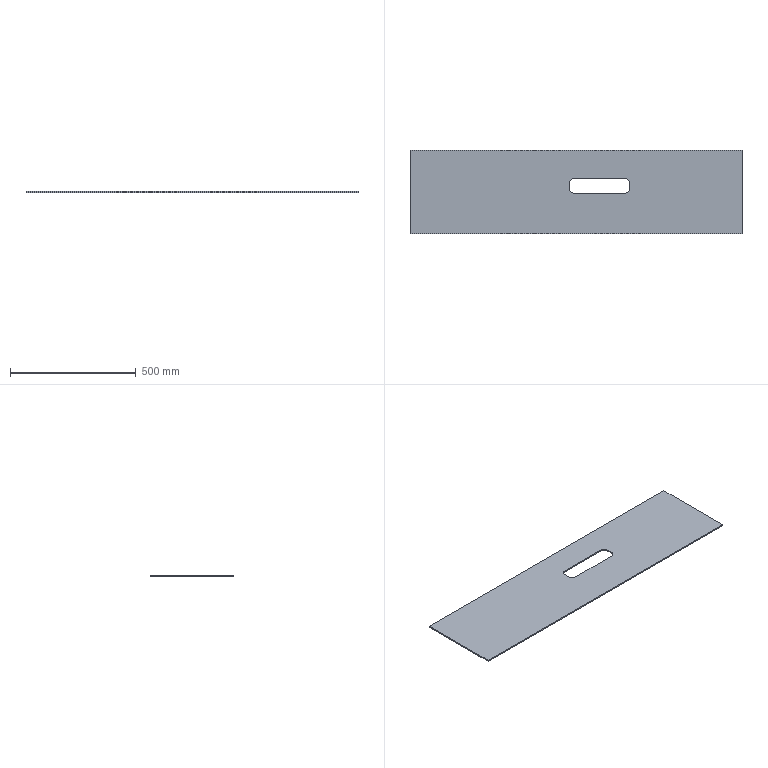Part | STEP file | 1 solid | 14 faces | box 1318 x 331 x 5 mm | volume 2111007 mm3 | plane 10 | cylinder 4 | commonest cylinder face diameters 40 x4
STEP:
#1=CARTESIAN_POINT('',(0.,0.,0.));
#2=DIRECTION('',(0.,0.,1.));
#3=DIRECTION('',(1.,0.,0.));
#4=AXIS2_PLACEMENT_3D('',#1,#2,#3);
#5=CARTESIAN_POINT('',(-7.,1028.,0.));
#6=VERTEX_POINT('',#5);
#7=CARTESIAN_POINT('',(193.,1028.,0.));
#8=VERTEX_POINT('',#7);
#9=CARTESIAN_POINT('',(-7.,1028.,0.));
#10=DIRECTION('',(1.,0.,0.));
#11=VECTOR('',#10,1.);
#12=LINE('',#9,#11);
#13=CARTESIAN_POINT('',(0.,0.,0.));
#14=DIRECTION('',(0.,0.,1.));
#15=DIRECTION('',(1.,0.,0.));
#16=AXIS2_PLACEMENT_3D('',#13,#14,#15);
#17=PLANE('',#16);
#18=CARTESIAN_POINT('',(-7.,1028.));
#19=DIRECTION('',(1.,0.));
#20=VECTOR('',#19,1.);
#21=LINE('',#18,#20);
#22=(GEOMETRIC_REPRESENTATION_CONTEXT(2)PARAMETRIC_REPRESENTATION_CONTEXT()REPRESENTATION_CONTEXT('',''));
#23=DEFINITIONAL_REPRESENTATION('',(#21),#22);
#24=PCURVE('',#17,#23);
#25=CARTESIAN_POINT('',(-7.,1028.,5.));
#26=DIRECTION('',(0.,-1.,0.));
#27=DIRECTION('',(0.,0.,-1.));
#28=AXIS2_PLACEMENT_3D('',#25,#26,#27);
#29=PLANE('',#28);
#30=CARTESIAN_POINT('',(5.,0.));
#31=DIRECTION('',(0.,1.));
#32=VECTOR('',#31,1.);
#33=LINE('',#30,#32);
#34=(GEOMETRIC_REPRESENTATION_CONTEXT(2)PARAMETRIC_REPRESENTATION_CONTEXT()REPRESENTATION_CONTEXT('',''));
#35=DEFINITIONAL_REPRESENTATION('',(#33),#34);
#36=PCURVE('',#29,#35);
#37=SURFACE_CURVE('',#12,(#24,#36),.PCURVE_S1.);
#38=EDGE_CURVE('',#6,#8,#37,.T.);
#39=ORIENTED_EDGE('',*,*,#38,.F.);
#40=CARTESIAN_POINT('',(-27.,1008.,0.));
#41=VERTEX_POINT('',#40);
#42=CARTESIAN_POINT('',(-7.,1008.,0.));
#43=DIRECTION('',(0.,0.,1.));
#44=DIRECTION('',(-1.,0.,0.));
#45=AXIS2_PLACEMENT_3D('',#42,#43,#44);
#46=CIRCLE('',#45,20.);
#47=CARTESIAN_POINT('',(-7.,1008.));
#48=DIRECTION('',(-1.,0.));
#49=AXIS2_PLACEMENT_2D('',#47,#48);
#50=CIRCLE('',#49,20.);
#51=(GEOMETRIC_REPRESENTATION_CONTEXT(2)PARAMETRIC_REPRESENTATION_CONTEXT()REPRESENTATION_CONTEXT('',''));
#52=DEFINITIONAL_REPRESENTATION('',(#50),#51);
#53=PCURVE('',#17,#52);
#54=CARTESIAN_POINT('',(-7.,1008.,5.));
#55=DIRECTION('',(0.,0.,-1.));
#56=DIRECTION('',(-1.,0.,0.));
#57=AXIS2_PLACEMENT_3D('',#54,#55,#56);
#58=CYLINDRICAL_SURFACE('',#57,20.);
#59=CARTESIAN_POINT('',(6.283,5.));
#60=DIRECTION('',(-1.,0.));
#61=VECTOR('',#60,1.);
#62=LINE('',#59,#61);
#63=(GEOMETRIC_REPRESENTATION_CONTEXT(2)PARAMETRIC_REPRESENTATION_CONTEXT()REPRESENTATION_CONTEXT('',''));
#64=DEFINITIONAL_REPRESENTATION('',(#62),#63);
#65=PCURVE('',#58,#64);
#66=SURFACE_CURVE('',#46,(#53,#65),.PCURVE_S1.);
#67=EDGE_CURVE('',#6,#41,#66,.T.);
#68=ORIENTED_EDGE('',*,*,#67,.T.);
#69=CARTESIAN_POINT('',(-27.,988.,0.));
#70=VERTEX_POINT('',#69);
#71=CARTESIAN_POINT('',(-27.,988.,0.));
#72=DIRECTION('',(0.,1.,0.));
#73=VECTOR('',#72,1.);
#74=LINE('',#71,#73);
#75=CARTESIAN_POINT('',(-27.,988.));
#76=DIRECTION('',(0.,1.));
#77=VECTOR('',#76,1.);
#78=LINE('',#75,#77);
#79=(GEOMETRIC_REPRESENTATION_CONTEXT(2)PARAMETRIC_REPRESENTATION_CONTEXT()REPRESENTATION_CONTEXT('',''));
#80=DEFINITIONAL_REPRESENTATION('',(#78),#79);
#81=PCURVE('',#17,#80);
#82=CARTESIAN_POINT('',(-27.,988.,5.));
#83=DIRECTION('',(1.,0.,0.));
#84=DIRECTION('',(0.,1.,0.));
#85=AXIS2_PLACEMENT_3D('',#82,#83,#84);
#86=PLANE('',#85);
#87=CARTESIAN_POINT('',(0.,-5.));
#88=DIRECTION('',(1.,0.));
#89=VECTOR('',#88,1.);
#90=LINE('',#87,#89);
#91=(GEOMETRIC_REPRESENTATION_CONTEXT(2)PARAMETRIC_REPRESENTATION_CONTEXT()REPRESENTATION_CONTEXT('',''));
#92=DEFINITIONAL_REPRESENTATION('',(#90),#91);
#93=PCURVE('',#86,#92);
#94=SURFACE_CURVE('',#74,(#81,#93),.PCURVE_S1.);
#95=EDGE_CURVE('',#70,#41,#94,.T.);
#96=ORIENTED_EDGE('',*,*,#95,.F.);
#97=CARTESIAN_POINT('',(-7.,968.,0.));
#98=VERTEX_POINT('',#97);
#99=CARTESIAN_POINT('',(-7.,988.,0.));
#100=DIRECTION('',(0.,0.,1.));
#101=DIRECTION('',(-1.,0.,0.));
#102=AXIS2_PLACEMENT_3D('',#99,#100,#101);
#103=CIRCLE('',#102,20.);
#104=CARTESIAN_POINT('',(-7.,988.));
#105=DIRECTION('',(-1.,0.));
#106=AXIS2_PLACEMENT_2D('',#104,#105);
#107=CIRCLE('',#106,20.);
#108=(GEOMETRIC_REPRESENTATION_CONTEXT(2)PARAMETRIC_REPRESENTATION_CONTEXT()REPRESENTATION_CONTEXT('',''));
#109=DEFINITIONAL_REPRESENTATION('',(#107),#108);
#110=PCURVE('',#17,#109);
#111=CARTESIAN_POINT('',(-7.,988.,5.));
#112=DIRECTION('',(0.,0.,-1.));
#113=DIRECTION('',(-1.,0.,0.));
#114=AXIS2_PLACEMENT_3D('',#111,#112,#113);
#115=CYLINDRICAL_SURFACE('',#114,20.);
#116=CARTESIAN_POINT('',(6.283,5.));
#117=DIRECTION('',(-1.,0.));
#118=VECTOR('',#117,1.);
#119=LINE('',#116,#118);
#120=(GEOMETRIC_REPRESENTATION_CONTEXT(2)PARAMETRIC_REPRESENTATION_CONTEXT()REPRESENTATION_CONTEXT('',''));
#121=DEFINITIONAL_REPRESENTATION('',(#119),#120);
#122=PCURVE('',#115,#121);
#123=SURFACE_CURVE('',#103,(#110,#122),.PCURVE_S1.);
#124=EDGE_CURVE('',#70,#98,#123,.T.);
#125=ORIENTED_EDGE('',*,*,#124,.T.);
#126=CARTESIAN_POINT('',(193.,968.,0.));
#127=VERTEX_POINT('',#126);
#128=CARTESIAN_POINT('',(-7.,968.,0.));
#129=DIRECTION('',(-1.,0.,0.));
#130=VECTOR('',#129,1.);
#131=LINE('',#128,#130);
#132=CARTESIAN_POINT('',(-7.,968.));
#133=DIRECTION('',(-1.,0.));
#134=VECTOR('',#133,1.);
#135=LINE('',#132,#134);
#136=(GEOMETRIC_REPRESENTATION_CONTEXT(2)PARAMETRIC_REPRESENTATION_CONTEXT()REPRESENTATION_CONTEXT('',''));
#137=DEFINITIONAL_REPRESENTATION('',(#135),#136);
#138=PCURVE('',#17,#137);
#139=CARTESIAN_POINT('',(-7.,968.,5.));
#140=DIRECTION('',(0.,1.,0.));
#141=DIRECTION('',(1.,0.,0.));
#142=AXIS2_PLACEMENT_3D('',#139,#140,#141);
#143=PLANE('',#142);
#144=CARTESIAN_POINT('',(0.,5.));
#145=DIRECTION('',(-1.,0.));
#146=VECTOR('',#145,1.);
#147=LINE('',#144,#146);
#148=(GEOMETRIC_REPRESENTATION_CONTEXT(2)PARAMETRIC_REPRESENTATION_CONTEXT()REPRESENTATION_CONTEXT('',''));
#149=DEFINITIONAL_REPRESENTATION('',(#147),#148);
#150=PCURVE('',#143,#149);
#151=SURFACE_CURVE('',#131,(#138,#150),.PCURVE_S1.);
#152=EDGE_CURVE('',#127,#98,#151,.T.);
#153=ORIENTED_EDGE('',*,*,#152,.F.);
#154=CARTESIAN_POINT('',(213.,988.,0.));
#155=VERTEX_POINT('',#154);
#156=CARTESIAN_POINT('',(193.,988.,0.));
#157=DIRECTION('',(0.,0.,1.));
#158=DIRECTION('',(-1.,0.,0.));
#159=AXIS2_PLACEMENT_3D('',#156,#157,#158);
#160=CIRCLE('',#159,20.);
#161=CARTESIAN_POINT('',(193.,988.));
#162=DIRECTION('',(-1.,0.));
#163=AXIS2_PLACEMENT_2D('',#161,#162);
#164=CIRCLE('',#163,20.);
#165=(GEOMETRIC_REPRESENTATION_CONTEXT(2)PARAMETRIC_REPRESENTATION_CONTEXT()REPRESENTATION_CONTEXT('',''));
#166=DEFINITIONAL_REPRESENTATION('',(#164),#165);
#167=PCURVE('',#17,#166);
#168=CARTESIAN_POINT('',(193.,988.,5.));
#169=DIRECTION('',(0.,0.,-1.));
#170=DIRECTION('',(-1.,0.,0.));
#171=AXIS2_PLACEMENT_3D('',#168,#169,#170);
#172=CYLINDRICAL_SURFACE('',#171,20.);
#173=CARTESIAN_POINT('',(6.283,5.));
#174=DIRECTION('',(-1.,0.));
#175=VECTOR('',#174,1.);
#176=LINE('',#173,#175);
#177=(GEOMETRIC_REPRESENTATION_CONTEXT(2)PARAMETRIC_REPRESENTATION_CONTEXT()REPRESENTATION_CONTEXT('',''));
#178=DEFINITIONAL_REPRESENTATION('',(#176),#177);
#179=PCURVE('',#172,#178);
#180=SURFACE_CURVE('',#160,(#167,#179),.PCURVE_S1.);
#181=EDGE_CURVE('',#127,#155,#180,.T.);
#182=ORIENTED_EDGE('',*,*,#181,.T.);
#183=CARTESIAN_POINT('',(213.,1008.,0.));
#184=VERTEX_POINT('',#183);
#185=CARTESIAN_POINT('',(213.,988.,0.));
#186=DIRECTION('',(0.,-1.,0.));
#187=VECTOR('',#186,1.);
#188=LINE('',#185,#187);
#189=CARTESIAN_POINT('',(213.,988.));
#190=DIRECTION('',(0.,-1.));
#191=VECTOR('',#190,1.);
#192=LINE('',#189,#191);
#193=(GEOMETRIC_REPRESENTATION_CONTEXT(2)PARAMETRIC_REPRESENTATION_CONTEXT()REPRESENTATION_CONTEXT('',''));
#194=DEFINITIONAL_REPRESENTATION('',(#192),#193);
#195=PCURVE('',#17,#194);
#196=CARTESIAN_POINT('',(213.,988.,5.));
#197=DIRECTION('',(-1.,0.,0.));
#198=DIRECTION('',(0.,0.,1.));
#199=AXIS2_PLACEMENT_3D('',#196,#197,#198);
#200=PLANE('',#199);
#201=CARTESIAN_POINT('',(-5.,0.));
#202=DIRECTION('',(0.,-1.));
#203=VECTOR('',#202,1.);
#204=LINE('',#201,#203);
#205=(GEOMETRIC_REPRESENTATION_CONTEXT(2)PARAMETRIC_REPRESENTATION_CONTEXT()REPRESENTATION_CONTEXT('',''));
#206=DEFINITIONAL_REPRESENTATION('',(#204),#205);
#207=PCURVE('',#200,#206);
#208=SURFACE_CURVE('',#188,(#195,#207),.PCURVE_S1.);
#209=EDGE_CURVE('',#184,#155,#208,.T.);
#210=ORIENTED_EDGE('',*,*,#209,.F.);
#211=CARTESIAN_POINT('',(193.,1008.,0.));
#212=DIRECTION('',(0.,0.,1.));
#213=DIRECTION('',(-1.,0.,0.));
#214=AXIS2_PLACEMENT_3D('',#211,#212,#213);
#215=CIRCLE('',#214,20.);
#216=CARTESIAN_POINT('',(193.,1008.));
#217=DIRECTION('',(-1.,0.));
#218=AXIS2_PLACEMENT_2D('',#216,#217);
#219=CIRCLE('',#218,20.);
#220=(GEOMETRIC_REPRESENTATION_CONTEXT(2)PARAMETRIC_REPRESENTATION_CONTEXT()REPRESENTATION_CONTEXT('',''));
#221=DEFINITIONAL_REPRESENTATION('',(#219),#220);
#222=PCURVE('',#17,#221);
#223=CARTESIAN_POINT('',(193.,1008.,5.));
#224=DIRECTION('',(0.,0.,-1.));
#225=DIRECTION('',(-1.,0.,0.));
#226=AXIS2_PLACEMENT_3D('',#223,#224,#225);
#227=CYLINDRICAL_SURFACE('',#226,20.);
#228=CARTESIAN_POINT('',(6.283,5.));
#229=DIRECTION('',(-1.,0.));
#230=VECTOR('',#229,1.);
#231=LINE('',#228,#230);
#232=(GEOMETRIC_REPRESENTATION_CONTEXT(2)PARAMETRIC_REPRESENTATION_CONTEXT()REPRESENTATION_CONTEXT('',''));
#233=DEFINITIONAL_REPRESENTATION('',(#231),#232);
#234=PCURVE('',#227,#233);
#235=SURFACE_CURVE('',#215,(#222,#234),.PCURVE_S1.);
#236=EDGE_CURVE('',#184,#8,#235,.T.);
#237=ORIENTED_EDGE('',*,*,#236,.T.);
#238=EDGE_LOOP('',(#39,#68,#96,#125,#153,#182,#210,#237));
#239=FACE_BOUND('',#238,.T.);
#240=CARTESIAN_POINT('',(-659.,808.,0.));
#241=VERTEX_POINT('',#240);
#242=CARTESIAN_POINT('',(-659.,1139.,0.));
#243=VERTEX_POINT('',#242);
#244=CARTESIAN_POINT('',(-659.,1139.,0.));
#245=DIRECTION('',(0.,1.,0.));
#246=VECTOR('',#245,1.);
#247=LINE('',#244,#246);
#248=CARTESIAN_POINT('',(-659.,1139.));
#249=DIRECTION('',(0.,1.));
#250=VECTOR('',#249,1.);
#251=LINE('',#248,#250);
#252=(GEOMETRIC_REPRESENTATION_CONTEXT(2)PARAMETRIC_REPRESENTATION_CONTEXT()REPRESENTATION_CONTEXT('',''));
#253=DEFINITIONAL_REPRESENTATION('',(#251),#252);
#254=PCURVE('',#17,#253);
#255=CARTESIAN_POINT('',(-659.,1139.,5.));
#256=DIRECTION('',(1.,0.,0.));
#257=DIRECTION('',(0.,1.,0.));
#258=AXIS2_PLACEMENT_3D('',#255,#256,#257);
#259=PLANE('',#258);
#260=CARTESIAN_POINT('',(0.,-5.));
#261=DIRECTION('',(1.,0.));
#262=VECTOR('',#261,1.);
#263=LINE('',#260,#262);
#264=(GEOMETRIC_REPRESENTATION_CONTEXT(2)PARAMETRIC_REPRESENTATION_CONTEXT()REPRESENTATION_CONTEXT('',''));
#265=DEFINITIONAL_REPRESENTATION('',(#263),#264);
#266=PCURVE('',#259,#265);
#267=SURFACE_CURVE('',#247,(#254,#266),.PCURVE_S1.);
#268=EDGE_CURVE('',#241,#243,#267,.T.);
#269=ORIENTED_EDGE('',*,*,#268,.T.);
#270=CARTESIAN_POINT('',(659.,1139.,0.));
#271=VERTEX_POINT('',#270);
#272=CARTESIAN_POINT('',(659.,1139.,0.));
#273=DIRECTION('',(1.,0.,0.));
#274=VECTOR('',#273,1.);
#275=LINE('',#272,#274);
#276=CARTESIAN_POINT('',(659.,1139.));
#277=DIRECTION('',(1.,0.));
#278=VECTOR('',#277,1.);
#279=LINE('',#276,#278);
#280=(GEOMETRIC_REPRESENTATION_CONTEXT(2)PARAMETRIC_REPRESENTATION_CONTEXT()REPRESENTATION_CONTEXT('',''));
#281=DEFINITIONAL_REPRESENTATION('',(#279),#280);
#282=PCURVE('',#17,#281);
#283=CARTESIAN_POINT('',(659.,1139.,5.));
#284=DIRECTION('',(0.,-1.,0.));
#285=DIRECTION('',(0.,0.,-1.));
#286=AXIS2_PLACEMENT_3D('',#283,#284,#285);
#287=PLANE('',#286);
#288=CARTESIAN_POINT('',(5.,0.));
#289=DIRECTION('',(0.,1.));
#290=VECTOR('',#289,1.);
#291=LINE('',#288,#290);
#292=(GEOMETRIC_REPRESENTATION_CONTEXT(2)PARAMETRIC_REPRESENTATION_CONTEXT()REPRESENTATION_CONTEXT('',''));
#293=DEFINITIONAL_REPRESENTATION('',(#291),#292);
#294=PCURVE('',#287,#293);
#295=SURFACE_CURVE('',#275,(#282,#294),.PCURVE_S1.);
#296=EDGE_CURVE('',#243,#271,#295,.T.);
#297=ORIENTED_EDGE('',*,*,#296,.T.);
#298=CARTESIAN_POINT('',(659.,808.,0.));
#299=VERTEX_POINT('',#298);
#300=CARTESIAN_POINT('',(659.,808.,0.));
#301=DIRECTION('',(0.,-1.,0.));
#302=VECTOR('',#301,1.);
#303=LINE('',#300,#302);
#304=CARTESIAN_POINT('',(659.,808.));
#305=DIRECTION('',(0.,-1.));
#306=VECTOR('',#305,1.);
#307=LINE('',#304,#306);
#308=(GEOMETRIC_REPRESENTATION_CONTEXT(2)PARAMETRIC_REPRESENTATION_CONTEXT()REPRESENTATION_CONTEXT('',''));
#309=DEFINITIONAL_REPRESENTATION('',(#307),#308);
#310=PCURVE('',#17,#309);
#311=CARTESIAN_POINT('',(659.,808.,5.));
#312=DIRECTION('',(-1.,0.,0.));
#313=DIRECTION('',(0.,1.,0.));
#314=AXIS2_PLACEMENT_3D('',#311,#312,#313);
#315=PLANE('',#314);
#316=CARTESIAN_POINT('',(0.,5.));
#317=DIRECTION('',(-1.,0.));
#318=VECTOR('',#317,1.);
#319=LINE('',#316,#318);
#320=(GEOMETRIC_REPRESENTATION_CONTEXT(2)PARAMETRIC_REPRESENTATION_CONTEXT()REPRESENTATION_CONTEXT('',''));
#321=DEFINITIONAL_REPRESENTATION('',(#319),#320);
#322=PCURVE('',#315,#321);
#323=SURFACE_CURVE('',#303,(#310,#322),.PCURVE_S1.);
#324=EDGE_CURVE('',#271,#299,#323,.T.);
#325=ORIENTED_EDGE('',*,*,#324,.T.);
#326=CARTESIAN_POINT('',(-659.,808.,0.));
#327=DIRECTION('',(-1.,0.,0.));
#328=VECTOR('',#327,1.);
#329=LINE('',#326,#328);
#330=CARTESIAN_POINT('',(-659.,808.));
#331=DIRECTION('',(-1.,0.));
#332=VECTOR('',#331,1.);
#333=LINE('',#330,#332);
#334=(GEOMETRIC_REPRESENTATION_CONTEXT(2)PARAMETRIC_REPRESENTATION_CONTEXT()REPRESENTATION_CONTEXT('',''));
#335=DEFINITIONAL_REPRESENTATION('',(#333),#334);
#336=PCURVE('',#17,#335);
#337=CARTESIAN_POINT('',(-659.,808.,5.));
#338=DIRECTION('',(0.,1.,0.));
#339=DIRECTION('',(1.,0.,0.));
#340=AXIS2_PLACEMENT_3D('',#337,#338,#339);
#341=PLANE('',#340);
#342=CARTESIAN_POINT('',(0.,5.));
#343=DIRECTION('',(-1.,0.));
#344=VECTOR('',#343,1.);
#345=LINE('',#342,#344);
#346=(GEOMETRIC_REPRESENTATION_CONTEXT(2)PARAMETRIC_REPRESENTATION_CONTEXT()REPRESENTATION_CONTEXT('',''));
#347=DEFINITIONAL_REPRESENTATION('',(#345),#346);
#348=PCURVE('',#341,#347);
#349=SURFACE_CURVE('',#329,(#336,#348),.PCURVE_S1.);
#350=EDGE_CURVE('',#299,#241,#349,.T.);
#351=ORIENTED_EDGE('',*,*,#350,.T.);
#352=EDGE_LOOP('',(#269,#297,#325,#351));
#353=FACE_BOUND('',#352,.T.);
#354=ADVANCED_FACE('',(#239,#353),#17,.F.);
#355=CARTESIAN_POINT('',(659.,808.,5.));
#356=VERTEX_POINT('',#355);
#357=CARTESIAN_POINT('',(659.,808.,5.));
#358=DIRECTION('',(0.,0.,1.));
#359=VECTOR('',#358,1.);
#360=LINE('',#357,#359);
#361=CARTESIAN_POINT('',(1318.,0.));
#362=DIRECTION('',(0.,-1.));
#363=VECTOR('',#362,1.);
#364=LINE('',#361,#363);
#365=(GEOMETRIC_REPRESENTATION_CONTEXT(2)PARAMETRIC_REPRESENTATION_CONTEXT()REPRESENTATION_CONTEXT('',''));
#366=DEFINITIONAL_REPRESENTATION('',(#364),#365);
#367=PCURVE('',#341,#366);
#368=CARTESIAN_POINT('',(0.,0.));
#369=DIRECTION('',(0.,-1.));
#370=VECTOR('',#369,1.);
#371=LINE('',#368,#370);
#372=(GEOMETRIC_REPRESENTATION_CONTEXT(2)PARAMETRIC_REPRESENTATION_CONTEXT()REPRESENTATION_CONTEXT('',''));
#373=DEFINITIONAL_REPRESENTATION('',(#371),#372);
#374=PCURVE('',#315,#373);
#375=SURFACE_CURVE('',#360,(#367,#374),.PCURVE_S1.);
#376=EDGE_CURVE('',#299,#356,#375,.T.);
#377=ORIENTED_EDGE('',*,*,#376,.T.);
#378=CARTESIAN_POINT('',(-659.,808.,5.));
#379=VERTEX_POINT('',#378);
#380=CARTESIAN_POINT('',(0.,808.,5.));
#381=DIRECTION('',(1.,0.,0.));
#382=VECTOR('',#381,1.);
#383=LINE('',#380,#382);
#384=CARTESIAN_POINT('',(659.,0.));
#385=DIRECTION('',(1.,0.));
#386=VECTOR('',#385,1.);
#387=LINE('',#384,#386);
#388=(GEOMETRIC_REPRESENTATION_CONTEXT(2)PARAMETRIC_REPRESENTATION_CONTEXT()REPRESENTATION_CONTEXT('',''));
#389=DEFINITIONAL_REPRESENTATION('',(#387),#388);
#390=PCURVE('',#341,#389);
#391=CARTESIAN_POINT('',(0.,0.,5.));
#392=DIRECTION('',(0.,0.,1.));
#393=DIRECTION('',(1.,0.,0.));
#394=AXIS2_PLACEMENT_3D('',#391,#392,#393);
#395=PLANE('',#394);
#396=CARTESIAN_POINT('',(0.,808.));
#397=DIRECTION('',(1.,0.));
#398=VECTOR('',#397,1.);
#399=LINE('',#396,#398);
#400=(GEOMETRIC_REPRESENTATION_CONTEXT(2)PARAMETRIC_REPRESENTATION_CONTEXT()REPRESENTATION_CONTEXT('',''));
#401=DEFINITIONAL_REPRESENTATION('',(#399),#400);
#402=PCURVE('',#395,#401);
#403=SURFACE_CURVE('',#383,(#390,#402),.PCURVE_S1.);
#404=EDGE_CURVE('',#379,#356,#403,.T.);
#405=ORIENTED_EDGE('',*,*,#404,.F.);
#406=CARTESIAN_POINT('',(-659.,808.,5.));
#407=DIRECTION('',(0.,0.,-1.));
#408=VECTOR('',#407,1.);
#409=LINE('',#406,#408);
#410=CARTESIAN_POINT('',(0.,0.));
#411=DIRECTION('',(0.,1.));
#412=VECTOR('',#411,1.);
#413=LINE('',#410,#412);
#414=(GEOMETRIC_REPRESENTATION_CONTEXT(2)PARAMETRIC_REPRESENTATION_CONTEXT()REPRESENTATION_CONTEXT('',''));
#415=DEFINITIONAL_REPRESENTATION('',(#413),#414);
#416=PCURVE('',#341,#415);
#417=CARTESIAN_POINT('',(-331.,0.));
#418=DIRECTION('',(0.,-1.));
#419=VECTOR('',#418,1.);
#420=LINE('',#417,#419);
#421=(GEOMETRIC_REPRESENTATION_CONTEXT(2)PARAMETRIC_REPRESENTATION_CONTEXT()REPRESENTATION_CONTEXT('',''));
#422=DEFINITIONAL_REPRESENTATION('',(#420),#421);
#423=PCURVE('',#259,#422);
#424=SURFACE_CURVE('',#409,(#416,#423),.PCURVE_S1.);
#425=EDGE_CURVE('',#379,#241,#424,.T.);
#426=ORIENTED_EDGE('',*,*,#425,.T.);
#427=ORIENTED_EDGE('',*,*,#350,.F.);
#428=EDGE_LOOP('',(#377,#405,#426,#427));
#429=FACE_BOUND('',#428,.T.);
#430=ADVANCED_FACE('',(#429),#341,.F.);
#431=CARTESIAN_POINT('',(659.,1139.,5.));
#432=VERTEX_POINT('',#431);
#433=CARTESIAN_POINT('',(659.,1139.,5.));
#434=DIRECTION('',(0.,0.,1.));
#435=VECTOR('',#434,1.);
#436=LINE('',#433,#435);
#437=CARTESIAN_POINT('',(331.,0.));
#438=DIRECTION('',(0.,-1.));
#439=VECTOR('',#438,1.);
#440=LINE('',#437,#439);
#441=(GEOMETRIC_REPRESENTATION_CONTEXT(2)PARAMETRIC_REPRESENTATION_CONTEXT()REPRESENTATION_CONTEXT('',''));
#442=DEFINITIONAL_REPRESENTATION('',(#440),#441);
#443=PCURVE('',#315,#442);
#444=CARTESIAN_POINT('',(0.,0.));
#445=DIRECTION('',(-1.,0.));
#446=VECTOR('',#445,1.);
#447=LINE('',#444,#446);
#448=(GEOMETRIC_REPRESENTATION_CONTEXT(2)PARAMETRIC_REPRESENTATION_CONTEXT()REPRESENTATION_CONTEXT('',''));
#449=DEFINITIONAL_REPRESENTATION('',(#447),#448);
#450=PCURVE('',#287,#449);
#451=SURFACE_CURVE('',#436,(#443,#450),.PCURVE_S1.);
#452=EDGE_CURVE('',#271,#432,#451,.T.);
#453=ORIENTED_EDGE('',*,*,#452,.T.);
#454=CARTESIAN_POINT('',(659.,0.,5.));
#455=DIRECTION('',(0.,1.,0.));
#456=VECTOR('',#455,1.);
#457=LINE('',#454,#456);
#458=CARTESIAN_POINT('',(-808.,0.));
#459=DIRECTION('',(1.,0.));
#460=VECTOR('',#459,1.);
#461=LINE('',#458,#460);
#462=(GEOMETRIC_REPRESENTATION_CONTEXT(2)PARAMETRIC_REPRESENTATION_CONTEXT()REPRESENTATION_CONTEXT('',''));
#463=DEFINITIONAL_REPRESENTATION('',(#461),#462);
#464=PCURVE('',#315,#463);
#465=CARTESIAN_POINT('',(659.,0.));
#466=DIRECTION('',(0.,1.));
#467=VECTOR('',#466,1.);
#468=LINE('',#465,#467);
#469=(GEOMETRIC_REPRESENTATION_CONTEXT(2)PARAMETRIC_REPRESENTATION_CONTEXT()REPRESENTATION_CONTEXT('',''));
#470=DEFINITIONAL_REPRESENTATION('',(#468),#469);
#471=PCURVE('',#395,#470);
#472=SURFACE_CURVE('',#457,(#464,#471),.PCURVE_S1.);
#473=EDGE_CURVE('',#356,#432,#472,.T.);
#474=ORIENTED_EDGE('',*,*,#473,.F.);
#475=ORIENTED_EDGE('',*,*,#376,.F.);
#476=ORIENTED_EDGE('',*,*,#324,.F.);
#477=EDGE_LOOP('',(#453,#474,#475,#476));
#478=FACE_BOUND('',#477,.T.);
#479=ADVANCED_FACE('',(#478),#315,.F.);
#480=CARTESIAN_POINT('',(-659.,1139.,5.));
#481=VERTEX_POINT('',#480);
#482=CARTESIAN_POINT('',(-659.,1139.,5.));
#483=DIRECTION('',(0.,0.,1.));
#484=VECTOR('',#483,1.);
#485=LINE('',#482,#484);
#486=CARTESIAN_POINT('',(0.,-1318.));
#487=DIRECTION('',(-1.,0.));
#488=VECTOR('',#487,1.);
#489=LINE('',#486,#488);
#490=(GEOMETRIC_REPRESENTATION_CONTEXT(2)PARAMETRIC_REPRESENTATION_CONTEXT()REPRESENTATION_CONTEXT('',''));
#491=DEFINITIONAL_REPRESENTATION('',(#489),#490);
#492=PCURVE('',#287,#491);
#493=CARTESIAN_POINT('',(0.,0.));
#494=DIRECTION('',(0.,1.));
#495=VECTOR('',#494,1.);
#496=LINE('',#493,#495);
#497=(GEOMETRIC_REPRESENTATION_CONTEXT(2)PARAMETRIC_REPRESENTATION_CONTEXT()REPRESENTATION_CONTEXT('',''));
#498=DEFINITIONAL_REPRESENTATION('',(#496),#497);
#499=PCURVE('',#259,#498);
#500=SURFACE_CURVE('',#485,(#492,#499),.PCURVE_S1.);
#501=EDGE_CURVE('',#243,#481,#500,.T.);
#502=ORIENTED_EDGE('',*,*,#501,.T.);
#503=CARTESIAN_POINT('',(0.,1139.,5.));
#504=DIRECTION('',(-1.,0.,0.));
#505=VECTOR('',#504,1.);
#506=LINE('',#503,#505);
#507=CARTESIAN_POINT('',(0.,-659.));
#508=DIRECTION('',(0.,-1.));
#509=VECTOR('',#508,1.);
#510=LINE('',#507,#509);
#511=(GEOMETRIC_REPRESENTATION_CONTEXT(2)PARAMETRIC_REPRESENTATION_CONTEXT()REPRESENTATION_CONTEXT('',''));
#512=DEFINITIONAL_REPRESENTATION('',(#510),#511);
#513=PCURVE('',#287,#512);
#514=CARTESIAN_POINT('',(0.,1139.));
#515=DIRECTION('',(-1.,0.));
#516=VECTOR('',#515,1.);
#517=LINE('',#514,#516);
#518=(GEOMETRIC_REPRESENTATION_CONTEXT(2)PARAMETRIC_REPRESENTATION_CONTEXT()REPRESENTATION_CONTEXT('',''));
#519=DEFINITIONAL_REPRESENTATION('',(#517),#518);
#520=PCURVE('',#395,#519);
#521=SURFACE_CURVE('',#506,(#513,#520),.PCURVE_S1.);
#522=EDGE_CURVE('',#432,#481,#521,.T.);
#523=ORIENTED_EDGE('',*,*,#522,.F.);
#524=ORIENTED_EDGE('',*,*,#452,.F.);
#525=ORIENTED_EDGE('',*,*,#296,.F.);
#526=EDGE_LOOP('',(#502,#523,#524,#525));
#527=FACE_BOUND('',#526,.T.);
#528=ADVANCED_FACE('',(#527),#287,.F.);
#529=ORIENTED_EDGE('',*,*,#425,.F.);
#530=CARTESIAN_POINT('',(-659.,0.,5.));
#531=DIRECTION('',(0.,-1.,0.));
#532=VECTOR('',#531,1.);
#533=LINE('',#530,#532);
#534=CARTESIAN_POINT('',(-1139.,0.));
#535=DIRECTION('',(-1.,0.));
#536=VECTOR('',#535,1.);
#537=LINE('',#534,#536);
#538=(GEOMETRIC_REPRESENTATION_CONTEXT(2)PARAMETRIC_REPRESENTATION_CONTEXT()REPRESENTATION_CONTEXT('',''));
#539=DEFINITIONAL_REPRESENTATION('',(#537),#538);
#540=PCURVE('',#259,#539);
#541=CARTESIAN_POINT('',(-659.,0.));
#542=DIRECTION('',(0.,-1.));
#543=VECTOR('',#542,1.);
#544=LINE('',#541,#543);
#545=(GEOMETRIC_REPRESENTATION_CONTEXT(2)PARAMETRIC_REPRESENTATION_CONTEXT()REPRESENTATION_CONTEXT('',''));
#546=DEFINITIONAL_REPRESENTATION('',(#544),#545);
#547=PCURVE('',#395,#546);
#548=SURFACE_CURVE('',#533,(#540,#547),.PCURVE_S1.);
#549=EDGE_CURVE('',#481,#379,#548,.T.);
#550=ORIENTED_EDGE('',*,*,#549,.F.);
#551=ORIENTED_EDGE('',*,*,#501,.F.);
#552=ORIENTED_EDGE('',*,*,#268,.F.);
#553=EDGE_LOOP('',(#529,#550,#551,#552));
#554=FACE_BOUND('',#553,.T.);
#555=ADVANCED_FACE('',(#554),#259,.F.);
#556=CARTESIAN_POINT('',(-7.,1028.,5.));
#557=VERTEX_POINT('',#556);
#558=CARTESIAN_POINT('',(193.,1028.,5.));
#559=VERTEX_POINT('',#558);
#560=CARTESIAN_POINT('',(0.,1028.,5.));
#561=DIRECTION('',(1.,0.,0.));
#562=VECTOR('',#561,1.);
#563=LINE('',#560,#562);
#564=CARTESIAN_POINT('',(0.,7.));
#565=DIRECTION('',(0.,1.));
#566=VECTOR('',#565,1.);
#567=LINE('',#564,#566);
#568=(GEOMETRIC_REPRESENTATION_CONTEXT(2)PARAMETRIC_REPRESENTATION_CONTEXT()REPRESENTATION_CONTEXT('',''));
#569=DEFINITIONAL_REPRESENTATION('',(#567),#568);
#570=PCURVE('',#29,#569);
#571=CARTESIAN_POINT('',(0.,1028.));
#572=DIRECTION('',(1.,0.));
#573=VECTOR('',#572,1.);
#574=LINE('',#571,#573);
#575=(GEOMETRIC_REPRESENTATION_CONTEXT(2)PARAMETRIC_REPRESENTATION_CONTEXT()REPRESENTATION_CONTEXT('',''));
#576=DEFINITIONAL_REPRESENTATION('',(#574),#575);
#577=PCURVE('',#395,#576);
#578=SURFACE_CURVE('',#563,(#570,#577),.PCURVE_S1.);
#579=EDGE_CURVE('',#557,#559,#578,.T.);
#580=ORIENTED_EDGE('',*,*,#579,.F.);
#581=CARTESIAN_POINT('',(-7.,1028.,5.));
#582=DIRECTION('',(0.,0.,-1.));
#583=VECTOR('',#582,1.);
#584=LINE('',#581,#583);
#585=CARTESIAN_POINT('',(0.,0.));
#586=DIRECTION('',(1.,0.));
#587=VECTOR('',#586,1.);
#588=LINE('',#585,#587);
#589=(GEOMETRIC_REPRESENTATION_CONTEXT(2)PARAMETRIC_REPRESENTATION_CONTEXT()REPRESENTATION_CONTEXT('',''));
#590=DEFINITIONAL_REPRESENTATION('',(#588),#589);
#591=PCURVE('',#29,#590);
#592=CARTESIAN_POINT('',(1.571,0.));
#593=DIRECTION('',(0.,1.));
#594=VECTOR('',#593,1.);
#595=LINE('',#592,#594);
#596=(GEOMETRIC_REPRESENTATION_CONTEXT(2)PARAMETRIC_REPRESENTATION_CONTEXT()REPRESENTATION_CONTEXT('',''));
#597=DEFINITIONAL_REPRESENTATION('',(#595),#596);
#598=PCURVE('',#58,#597);
#599=SURFACE_CURVE('',#584,(#591,#598),.PCURVE_S1.);
#600=EDGE_CURVE('',#557,#6,#599,.T.);
#601=ORIENTED_EDGE('',*,*,#600,.T.);
#602=ORIENTED_EDGE('',*,*,#38,.T.);
#603=CARTESIAN_POINT('',(193.,1028.,5.));
#604=DIRECTION('',(0.,0.,1.));
#605=VECTOR('',#604,1.);
#606=LINE('',#603,#605);
#607=CARTESIAN_POINT('',(0.,200.));
#608=DIRECTION('',(-1.,0.));
#609=VECTOR('',#608,1.);
#610=LINE('',#607,#609);
#611=(GEOMETRIC_REPRESENTATION_CONTEXT(2)PARAMETRIC_REPRESENTATION_CONTEXT()REPRESENTATION_CONTEXT('',''));
#612=DEFINITIONAL_REPRESENTATION('',(#610),#611);
#613=PCURVE('',#29,#612);
#614=CARTESIAN_POINT('',(1.571,0.));
#615=DIRECTION('',(0.,-1.));
#616=VECTOR('',#615,1.);
#617=LINE('',#614,#616);
#618=(GEOMETRIC_REPRESENTATION_CONTEXT(2)PARAMETRIC_REPRESENTATION_CONTEXT()REPRESENTATION_CONTEXT('',''));
#619=DEFINITIONAL_REPRESENTATION('',(#617),#618);
#620=PCURVE('',#227,#619);
#621=SURFACE_CURVE('',#606,(#613,#620),.PCURVE_S1.);
#622=EDGE_CURVE('',#8,#559,#621,.T.);
#623=ORIENTED_EDGE('',*,*,#622,.T.);
#624=EDGE_LOOP('',(#580,#601,#602,#623));
#625=FACE_BOUND('',#624,.T.);
#626=ADVANCED_FACE('',(#625),#29,.T.);
#627=ORIENTED_EDGE('',*,*,#236,.T.);
#628=ORIENTED_EDGE('',*,*,#622,.T.);
#629=CARTESIAN_POINT('',(213.,1008.,5.));
#630=VERTEX_POINT('',#629);
#631=CARTESIAN_POINT('',(193.,1008.,5.));
#632=DIRECTION('',(0.,0.,-1.));
#633=DIRECTION('',(-1.,0.,0.));
#634=AXIS2_PLACEMENT_3D('',#631,#632,#633);
#635=CIRCLE('',#634,20.);
#636=CARTESIAN_POINT('',(0.,0.));
#637=DIRECTION('',(1.,0.));
#638=VECTOR('',#637,1.);
#639=LINE('',#636,#638);
#640=(GEOMETRIC_REPRESENTATION_CONTEXT(2)PARAMETRIC_REPRESENTATION_CONTEXT()REPRESENTATION_CONTEXT('',''));
#641=DEFINITIONAL_REPRESENTATION('',(#639),#640);
#642=PCURVE('',#227,#641);
#643=CARTESIAN_POINT('',(173.,1008.));
#644=CARTESIAN_POINT('',(173.,1042.641));
#645=CARTESIAN_POINT('',(203.,1025.321));
#646=CARTESIAN_POINT('',(233.,1008.));
#647=CARTESIAN_POINT('',(203.,990.679));
#648=CARTESIAN_POINT('',(173.,973.359));
#649=CARTESIAN_POINT('',(173.,1008.));
#650=(BOUNDED_CURVE()B_SPLINE_CURVE(2,(#643,#644,#645,#646,#647,#648,#649),.UNSPECIFIED.,.T.,.F.)B_SPLINE_CURVE_WITH_KNOTS((1,2,2,2,2,1),(-2.094,0.,2.094,4.189,6.283,8.378),.UNSPECIFIED.)CURVE()GEOMETRIC_REPRESENTATION_ITEM()RATIONAL_B_SPLINE_CURVE((1.,0.5,1.,0.5,1.,0.5,1.))REPRESENTATION_ITEM(''));
#651=(GEOMETRIC_REPRESENTATION_CONTEXT(2)PARAMETRIC_REPRESENTATION_CONTEXT()REPRESENTATION_CONTEXT('',''));
#652=DEFINITIONAL_REPRESENTATION('',(#650),#651);
#653=PCURVE('',#395,#652);
#654=SURFACE_CURVE('',#635,(#642,#653),.PCURVE_S1.);
#655=EDGE_CURVE('',#559,#630,#654,.T.);
#656=ORIENTED_EDGE('',*,*,#655,.T.);
#657=CARTESIAN_POINT('',(213.,1008.,5.));
#658=DIRECTION('',(0.,0.,-1.));
#659=VECTOR('',#658,1.);
#660=LINE('',#657,#659);
#661=CARTESIAN_POINT('',(3.142,0.));
#662=DIRECTION('',(0.,1.));
#663=VECTOR('',#662,1.);
#664=LINE('',#661,#663);
#665=(GEOMETRIC_REPRESENTATION_CONTEXT(2)PARAMETRIC_REPRESENTATION_CONTEXT()REPRESENTATION_CONTEXT('',''));
#666=DEFINITIONAL_REPRESENTATION('',(#664),#665);
#667=PCURVE('',#227,#666);
#668=CARTESIAN_POINT('',(0.,20.));
#669=DIRECTION('',(-1.,0.));
#670=VECTOR('',#669,1.);
#671=LINE('',#668,#670);
#672=(GEOMETRIC_REPRESENTATION_CONTEXT(2)PARAMETRIC_REPRESENTATION_CONTEXT()REPRESENTATION_CONTEXT('',''));
#673=DEFINITIONAL_REPRESENTATION('',(#671),#672);
#674=PCURVE('',#200,#673);
#675=SURFACE_CURVE('',#660,(#667,#674),.PCURVE_S1.);
#676=EDGE_CURVE('',#630,#184,#675,.T.);
#677=ORIENTED_EDGE('',*,*,#676,.T.);
#678=EDGE_LOOP('',(#627,#628,#656,#677));
#679=FACE_BOUND('',#678,.F.);
#680=ADVANCED_FACE('',(#679),#227,.F.);
#681=CARTESIAN_POINT('',(213.,988.,5.));
#682=VERTEX_POINT('',#681);
#683=CARTESIAN_POINT('',(213.,0.,5.));
#684=DIRECTION('',(0.,-1.,0.));
#685=VECTOR('',#684,1.);
#686=LINE('',#683,#685);
#687=CARTESIAN_POINT('',(0.,-988.));
#688=DIRECTION('',(0.,-1.));
#689=VECTOR('',#688,1.);
#690=LINE('',#687,#689);
#691=(GEOMETRIC_REPRESENTATION_CONTEXT(2)PARAMETRIC_REPRESENTATION_CONTEXT()REPRESENTATION_CONTEXT('',''));
#692=DEFINITIONAL_REPRESENTATION('',(#690),#691);
#693=PCURVE('',#200,#692);
#694=CARTESIAN_POINT('',(213.,0.));
#695=DIRECTION('',(0.,-1.));
#696=VECTOR('',#695,1.);
#697=LINE('',#694,#696);
#698=(GEOMETRIC_REPRESENTATION_CONTEXT(2)PARAMETRIC_REPRESENTATION_CONTEXT()REPRESENTATION_CONTEXT('',''));
#699=DEFINITIONAL_REPRESENTATION('',(#697),#698);
#700=PCURVE('',#395,#699);
#701=SURFACE_CURVE('',#686,(#693,#700),.PCURVE_S1.);
#702=EDGE_CURVE('',#630,#682,#701,.T.);
#703=ORIENTED_EDGE('',*,*,#702,.F.);
#704=ORIENTED_EDGE('',*,*,#676,.T.);
#705=ORIENTED_EDGE('',*,*,#209,.T.);
#706=CARTESIAN_POINT('',(213.,988.,5.));
#707=DIRECTION('',(0.,0.,1.));
#708=VECTOR('',#707,1.);
#709=LINE('',#706,#708);
#710=CARTESIAN_POINT('',(0.,0.));
#711=DIRECTION('',(1.,0.));
#712=VECTOR('',#711,1.);
#713=LINE('',#710,#712);
#714=(GEOMETRIC_REPRESENTATION_CONTEXT(2)PARAMETRIC_REPRESENTATION_CONTEXT()REPRESENTATION_CONTEXT('',''));
#715=DEFINITIONAL_REPRESENTATION('',(#713),#714);
#716=PCURVE('',#200,#715);
#717=CARTESIAN_POINT('',(3.142,0.));
#718=DIRECTION('',(0.,-1.));
#719=VECTOR('',#718,1.);
#720=LINE('',#717,#719);
#721=(GEOMETRIC_REPRESENTATION_CONTEXT(2)PARAMETRIC_REPRESENTATION_CONTEXT()REPRESENTATION_CONTEXT('',''));
#722=DEFINITIONAL_REPRESENTATION('',(#720),#721);
#723=PCURVE('',#172,#722);
#724=SURFACE_CURVE('',#709,(#716,#723),.PCURVE_S1.);
#725=EDGE_CURVE('',#155,#682,#724,.T.);
#726=ORIENTED_EDGE('',*,*,#725,.T.);
#727=EDGE_LOOP('',(#703,#704,#705,#726));
#728=FACE_BOUND('',#727,.T.);
#729=ADVANCED_FACE('',(#728),#200,.T.);
#730=ORIENTED_EDGE('',*,*,#181,.T.);
#731=ORIENTED_EDGE('',*,*,#725,.T.);
#732=CARTESIAN_POINT('',(193.,968.,5.));
#733=VERTEX_POINT('',#732);
#734=CARTESIAN_POINT('',(193.,988.,5.));
#735=DIRECTION('',(0.,0.,-1.));
#736=DIRECTION('',(-1.,0.,0.));
#737=AXIS2_PLACEMENT_3D('',#734,#735,#736);
#738=CIRCLE('',#737,20.);
#739=CARTESIAN_POINT('',(0.,0.));
#740=DIRECTION('',(1.,0.));
#741=VECTOR('',#740,1.);
#742=LINE('',#739,#741);
#743=(GEOMETRIC_REPRESENTATION_CONTEXT(2)PARAMETRIC_REPRESENTATION_CONTEXT()REPRESENTATION_CONTEXT('',''));
#744=DEFINITIONAL_REPRESENTATION('',(#742),#743);
#745=PCURVE('',#172,#744);
#746=CARTESIAN_POINT('',(173.,988.));
#747=CARTESIAN_POINT('',(173.,1022.641));
#748=CARTESIAN_POINT('',(203.,1005.321));
#749=CARTESIAN_POINT('',(233.,988.));
#750=CARTESIAN_POINT('',(203.,970.679));
#751=CARTESIAN_POINT('',(173.,953.359));
#752=CARTESIAN_POINT('',(173.,988.));
#753=(BOUNDED_CURVE()B_SPLINE_CURVE(2,(#746,#747,#748,#749,#750,#751,#752),.UNSPECIFIED.,.T.,.F.)B_SPLINE_CURVE_WITH_KNOTS((1,2,2,2,2,1),(-2.094,0.,2.094,4.189,6.283,8.378),.UNSPECIFIED.)CURVE()GEOMETRIC_REPRESENTATION_ITEM()RATIONAL_B_SPLINE_CURVE((1.,0.5,1.,0.5,1.,0.5,1.))REPRESENTATION_ITEM(''));
#754=(GEOMETRIC_REPRESENTATION_CONTEXT(2)PARAMETRIC_REPRESENTATION_CONTEXT()REPRESENTATION_CONTEXT('',''));
#755=DEFINITIONAL_REPRESENTATION('',(#753),#754);
#756=PCURVE('',#395,#755);
#757=SURFACE_CURVE('',#738,(#745,#756),.PCURVE_S1.);
#758=EDGE_CURVE('',#682,#733,#757,.T.);
#759=ORIENTED_EDGE('',*,*,#758,.T.);
#760=CARTESIAN_POINT('',(193.,968.,5.));
#761=DIRECTION('',(0.,0.,-1.));
#762=VECTOR('',#761,1.);
#763=LINE('',#760,#762);
#764=CARTESIAN_POINT('',(4.712,0.));
#765=DIRECTION('',(0.,1.));
#766=VECTOR('',#765,1.);
#767=LINE('',#764,#766);
#768=(GEOMETRIC_REPRESENTATION_CONTEXT(2)PARAMETRIC_REPRESENTATION_CONTEXT()REPRESENTATION_CONTEXT('',''));
#769=DEFINITIONAL_REPRESENTATION('',(#767),#768);
#770=PCURVE('',#172,#769);
#771=CARTESIAN_POINT('',(200.,0.));
#772=DIRECTION('',(0.,1.));
#773=VECTOR('',#772,1.);
#774=LINE('',#771,#773);
#775=(GEOMETRIC_REPRESENTATION_CONTEXT(2)PARAMETRIC_REPRESENTATION_CONTEXT()REPRESENTATION_CONTEXT('',''));
#776=DEFINITIONAL_REPRESENTATION('',(#774),#775);
#777=PCURVE('',#143,#776);
#778=SURFACE_CURVE('',#763,(#770,#777),.PCURVE_S1.);
#779=EDGE_CURVE('',#733,#127,#778,.T.);
#780=ORIENTED_EDGE('',*,*,#779,.T.);
#781=EDGE_LOOP('',(#730,#731,#759,#780));
#782=FACE_BOUND('',#781,.F.);
#783=ADVANCED_FACE('',(#782),#172,.F.);
#784=CARTESIAN_POINT('',(-7.,968.,5.));
#785=VERTEX_POINT('',#784);
#786=CARTESIAN_POINT('',(0.,968.,5.));
#787=DIRECTION('',(-1.,0.,0.));
#788=VECTOR('',#787,1.);
#789=LINE('',#786,#788);
#790=CARTESIAN_POINT('',(7.,0.));
#791=DIRECTION('',(-1.,0.));
#792=VECTOR('',#791,1.);
#793=LINE('',#790,#792);
#794=(GEOMETRIC_REPRESENTATION_CONTEXT(2)PARAMETRIC_REPRESENTATION_CONTEXT()REPRESENTATION_CONTEXT('',''));
#795=DEFINITIONAL_REPRESENTATION('',(#793),#794);
#796=PCURVE('',#143,#795);
#797=CARTESIAN_POINT('',(0.,968.));
#798=DIRECTION('',(-1.,0.));
#799=VECTOR('',#798,1.);
#800=LINE('',#797,#799);
#801=(GEOMETRIC_REPRESENTATION_CONTEXT(2)PARAMETRIC_REPRESENTATION_CONTEXT()REPRESENTATION_CONTEXT('',''));
#802=DEFINITIONAL_REPRESENTATION('',(#800),#801);
#803=PCURVE('',#395,#802);
#804=SURFACE_CURVE('',#789,(#796,#803),.PCURVE_S1.);
#805=EDGE_CURVE('',#733,#785,#804,.T.);
#806=ORIENTED_EDGE('',*,*,#805,.F.);
#807=ORIENTED_EDGE('',*,*,#779,.T.);
#808=ORIENTED_EDGE('',*,*,#152,.T.);
#809=CARTESIAN_POINT('',(-7.,968.,5.));
#810=DIRECTION('',(0.,0.,1.));
#811=VECTOR('',#810,1.);
#812=LINE('',#809,#811);
#813=CARTESIAN_POINT('',(0.,0.));
#814=DIRECTION('',(0.,-1.));
#815=VECTOR('',#814,1.);
#816=LINE('',#813,#815);
#817=(GEOMETRIC_REPRESENTATION_CONTEXT(2)PARAMETRIC_REPRESENTATION_CONTEXT()REPRESENTATION_CONTEXT('',''));
#818=DEFINITIONAL_REPRESENTATION('',(#816),#817);
#819=PCURVE('',#143,#818);
#820=CARTESIAN_POINT('',(4.712,0.));
#821=DIRECTION('',(0.,-1.));
#822=VECTOR('',#821,1.);
#823=LINE('',#820,#822);
#824=(GEOMETRIC_REPRESENTATION_CONTEXT(2)PARAMETRIC_REPRESENTATION_CONTEXT()REPRESENTATION_CONTEXT('',''));
#825=DEFINITIONAL_REPRESENTATION('',(#823),#824);
#826=PCURVE('',#115,#825);
#827=SURFACE_CURVE('',#812,(#819,#826),.PCURVE_S1.);
#828=EDGE_CURVE('',#98,#785,#827,.T.);
#829=ORIENTED_EDGE('',*,*,#828,.T.);
#830=EDGE_LOOP('',(#806,#807,#808,#829));
#831=FACE_BOUND('',#830,.T.);
#832=ADVANCED_FACE('',(#831),#143,.T.);
#833=ORIENTED_EDGE('',*,*,#124,.T.);
#834=ORIENTED_EDGE('',*,*,#828,.T.);
#835=CARTESIAN_POINT('',(-27.,988.,5.));
#836=VERTEX_POINT('',#835);
#837=CARTESIAN_POINT('',(-7.,988.,5.));
#838=DIRECTION('',(0.,0.,-1.));
#839=DIRECTION('',(-1.,0.,0.));
#840=AXIS2_PLACEMENT_3D('',#837,#838,#839);
#841=CIRCLE('',#840,20.);
#842=CARTESIAN_POINT('',(0.,0.));
#843=DIRECTION('',(1.,0.));
#844=VECTOR('',#843,1.);
#845=LINE('',#842,#844);
#846=(GEOMETRIC_REPRESENTATION_CONTEXT(2)PARAMETRIC_REPRESENTATION_CONTEXT()REPRESENTATION_CONTEXT('',''));
#847=DEFINITIONAL_REPRESENTATION('',(#845),#846);
#848=PCURVE('',#115,#847);
#849=CARTESIAN_POINT('',(-27.,988.));
#850=CARTESIAN_POINT('',(-27.,1022.641));
#851=CARTESIAN_POINT('',(3.,1005.321));
#852=CARTESIAN_POINT('',(33.,988.));
#853=CARTESIAN_POINT('',(3.,970.679));
#854=CARTESIAN_POINT('',(-27.,953.359));
#855=CARTESIAN_POINT('',(-27.,988.));
#856=(BOUNDED_CURVE()B_SPLINE_CURVE(2,(#849,#850,#851,#852,#853,#854,#855),.UNSPECIFIED.,.T.,.F.)B_SPLINE_CURVE_WITH_KNOTS((1,2,2,2,2,1),(-2.094,0.,2.094,4.189,6.283,8.378),.UNSPECIFIED.)CURVE()GEOMETRIC_REPRESENTATION_ITEM()RATIONAL_B_SPLINE_CURVE((1.,0.5,1.,0.5,1.,0.5,1.))REPRESENTATION_ITEM(''));
#857=(GEOMETRIC_REPRESENTATION_CONTEXT(2)PARAMETRIC_REPRESENTATION_CONTEXT()REPRESENTATION_CONTEXT('',''));
#858=DEFINITIONAL_REPRESENTATION('',(#856),#857);
#859=PCURVE('',#395,#858);
#860=SURFACE_CURVE('',#841,(#848,#859),.PCURVE_S1.);
#861=EDGE_CURVE('',#785,#836,#860,.T.);
#862=ORIENTED_EDGE('',*,*,#861,.T.);
#863=CARTESIAN_POINT('',(-27.,988.,5.));
#864=DIRECTION('',(0.,0.,-1.));
#865=VECTOR('',#864,1.);
#866=LINE('',#863,#865);
#867=CARTESIAN_POINT('',(6.283,0.));
#868=DIRECTION('',(0.,1.));
#869=VECTOR('',#868,1.);
#870=LINE('',#867,#869);
#871=(GEOMETRIC_REPRESENTATION_CONTEXT(2)PARAMETRIC_REPRESENTATION_CONTEXT()REPRESENTATION_CONTEXT('',''));
#872=DEFINITIONAL_REPRESENTATION('',(#870),#871);
#873=PCURVE('',#115,#872);
#874=CARTESIAN_POINT('',(0.,0.));
#875=DIRECTION('',(0.,-1.));
#876=VECTOR('',#875,1.);
#877=LINE('',#874,#876);
#878=(GEOMETRIC_REPRESENTATION_CONTEXT(2)PARAMETRIC_REPRESENTATION_CONTEXT()REPRESENTATION_CONTEXT('',''));
#879=DEFINITIONAL_REPRESENTATION('',(#877),#878);
#880=PCURVE('',#86,#879);
#881=SURFACE_CURVE('',#866,(#873,#880),.PCURVE_S1.);
#882=EDGE_CURVE('',#836,#70,#881,.T.);
#883=ORIENTED_EDGE('',*,*,#882,.T.);
#884=EDGE_LOOP('',(#833,#834,#862,#883));
#885=FACE_BOUND('',#884,.F.);
#886=ADVANCED_FACE('',(#885),#115,.F.);
#887=CARTESIAN_POINT('',(-27.,1008.,5.));
#888=VERTEX_POINT('',#887);
#889=CARTESIAN_POINT('',(-27.,0.,5.));
#890=DIRECTION('',(0.,1.,0.));
#891=VECTOR('',#890,1.);
#892=LINE('',#889,#891);
#893=CARTESIAN_POINT('',(-988.,0.));
#894=DIRECTION('',(1.,0.));
#895=VECTOR('',#894,1.);
#896=LINE('',#893,#895);
#897=(GEOMETRIC_REPRESENTATION_CONTEXT(2)PARAMETRIC_REPRESENTATION_CONTEXT()REPRESENTATION_CONTEXT('',''));
#898=DEFINITIONAL_REPRESENTATION('',(#896),#897);
#899=PCURVE('',#86,#898);
#900=CARTESIAN_POINT('',(-27.,0.));
#901=DIRECTION('',(0.,1.));
#902=VECTOR('',#901,1.);
#903=LINE('',#900,#902);
#904=(GEOMETRIC_REPRESENTATION_CONTEXT(2)PARAMETRIC_REPRESENTATION_CONTEXT()REPRESENTATION_CONTEXT('',''));
#905=DEFINITIONAL_REPRESENTATION('',(#903),#904);
#906=PCURVE('',#395,#905);
#907=SURFACE_CURVE('',#892,(#899,#906),.PCURVE_S1.);
#908=EDGE_CURVE('',#836,#888,#907,.T.);
#909=ORIENTED_EDGE('',*,*,#908,.F.);
#910=ORIENTED_EDGE('',*,*,#882,.T.);
#911=ORIENTED_EDGE('',*,*,#95,.T.);
#912=CARTESIAN_POINT('',(-27.,1008.,5.));
#913=DIRECTION('',(0.,0.,1.));
#914=VECTOR('',#913,1.);
#915=LINE('',#912,#914);
#916=CARTESIAN_POINT('',(20.,0.));
#917=DIRECTION('',(0.,1.));
#918=VECTOR('',#917,1.);
#919=LINE('',#916,#918);
#920=(GEOMETRIC_REPRESENTATION_CONTEXT(2)PARAMETRIC_REPRESENTATION_CONTEXT()REPRESENTATION_CONTEXT('',''));
#921=DEFINITIONAL_REPRESENTATION('',(#919),#920);
#922=PCURVE('',#86,#921);
#923=CARTESIAN_POINT('',(0.,0.));
#924=DIRECTION('',(0.,-1.));
#925=VECTOR('',#924,1.);
#926=LINE('',#923,#925);
#927=(GEOMETRIC_REPRESENTATION_CONTEXT(2)PARAMETRIC_REPRESENTATION_CONTEXT()REPRESENTATION_CONTEXT('',''));
#928=DEFINITIONAL_REPRESENTATION('',(#926),#927);
#929=PCURVE('',#58,#928);
#930=SURFACE_CURVE('',#915,(#922,#929),.PCURVE_S1.);
#931=EDGE_CURVE('',#41,#888,#930,.T.);
#932=ORIENTED_EDGE('',*,*,#931,.T.);
#933=EDGE_LOOP('',(#909,#910,#911,#932));
#934=FACE_BOUND('',#933,.T.);
#935=ADVANCED_FACE('',(#934),#86,.T.);
#936=ORIENTED_EDGE('',*,*,#67,.T.);
#937=ORIENTED_EDGE('',*,*,#931,.T.);
#938=CARTESIAN_POINT('',(-7.,1008.,5.));
#939=DIRECTION('',(0.,0.,-1.));
#940=DIRECTION('',(-1.,0.,0.));
#941=AXIS2_PLACEMENT_3D('',#938,#939,#940);
#942=CIRCLE('',#941,20.);
#943=CARTESIAN_POINT('',(0.,0.));
#944=DIRECTION('',(1.,0.));
#945=VECTOR('',#944,1.);
#946=LINE('',#943,#945);
#947=(GEOMETRIC_REPRESENTATION_CONTEXT(2)PARAMETRIC_REPRESENTATION_CONTEXT()REPRESENTATION_CONTEXT('',''));
#948=DEFINITIONAL_REPRESENTATION('',(#946),#947);
#949=PCURVE('',#58,#948);
#950=CARTESIAN_POINT('',(-27.,1008.));
#951=CARTESIAN_POINT('',(-27.,1042.641));
#952=CARTESIAN_POINT('',(3.,1025.321));
#953=CARTESIAN_POINT('',(33.,1008.));
#954=CARTESIAN_POINT('',(3.,990.679));
#955=CARTESIAN_POINT('',(-27.,973.359));
#956=CARTESIAN_POINT('',(-27.,1008.));
#957=(BOUNDED_CURVE()B_SPLINE_CURVE(2,(#950,#951,#952,#953,#954,#955,#956),.UNSPECIFIED.,.T.,.F.)B_SPLINE_CURVE_WITH_KNOTS((1,2,2,2,2,1),(-2.094,0.,2.094,4.189,6.283,8.378),.UNSPECIFIED.)CURVE()GEOMETRIC_REPRESENTATION_ITEM()RATIONAL_B_SPLINE_CURVE((1.,0.5,1.,0.5,1.,0.5,1.))REPRESENTATION_ITEM(''));
#958=(GEOMETRIC_REPRESENTATION_CONTEXT(2)PARAMETRIC_REPRESENTATION_CONTEXT()REPRESENTATION_CONTEXT('',''));
#959=DEFINITIONAL_REPRESENTATION('',(#957),#958);
#960=PCURVE('',#395,#959);
#961=SURFACE_CURVE('',#942,(#949,#960),.PCURVE_S1.);
#962=EDGE_CURVE('',#888,#557,#961,.T.);
#963=ORIENTED_EDGE('',*,*,#962,.T.);
#964=ORIENTED_EDGE('',*,*,#600,.T.);
#965=EDGE_LOOP('',(#936,#937,#963,#964));
#966=FACE_BOUND('',#965,.F.);
#967=ADVANCED_FACE('',(#966),#58,.F.);
#968=ORIENTED_EDGE('',*,*,#908,.T.);
#969=ORIENTED_EDGE('',*,*,#962,.T.);
#970=ORIENTED_EDGE('',*,*,#579,.T.);
#971=ORIENTED_EDGE('',*,*,#655,.T.);
#972=ORIENTED_EDGE('',*,*,#702,.T.);
#973=ORIENTED_EDGE('',*,*,#758,.T.);
#974=ORIENTED_EDGE('',*,*,#805,.T.);
#975=ORIENTED_EDGE('',*,*,#861,.T.);
#976=EDGE_LOOP('',(#968,#969,#970,#971,#972,#973,#974,#975));
#977=FACE_BOUND('',#976,.T.);
#978=ORIENTED_EDGE('',*,*,#522,.T.);
#979=ORIENTED_EDGE('',*,*,#549,.T.);
#980=ORIENTED_EDGE('',*,*,#404,.T.);
#981=ORIENTED_EDGE('',*,*,#473,.T.);
#982=EDGE_LOOP('',(#978,#979,#980,#981));
#983=FACE_BOUND('',#982,.T.);
#984=ADVANCED_FACE('',(#977,#983),#395,.T.);
#985=CLOSED_SHELL('',(#354,#430,#479,#528,#555,#626,#680,#729,#783,#832,#886,#935,#967,#984));
#986=MANIFOLD_SOLID_BREP('',#985);
#987=(LENGTH_UNIT()NAMED_UNIT(*)SI_UNIT(.MILLI.,.METRE.));
#988=UNCERTAINTY_MEASURE_WITH_UNIT(LENGTH_MEASURE(0.0000001),#987,'','');
#989=(NAMED_UNIT(*)PLANE_ANGLE_UNIT()SI_UNIT($,.RADIAN.));
#990=(NAMED_UNIT(*)SI_UNIT($,.STERADIAN.)SOLID_ANGLE_UNIT());
#991=(GEOMETRIC_REPRESENTATION_CONTEXT(3)GLOBAL_UNCERTAINTY_ASSIGNED_CONTEXT((#988))GLOBAL_UNIT_ASSIGNED_CONTEXT((#987,#989,#990))REPRESENTATION_CONTEXT('',''));
#992=ADVANCED_BREP_SHAPE_REPRESENTATION('',(#4,#986),#991);